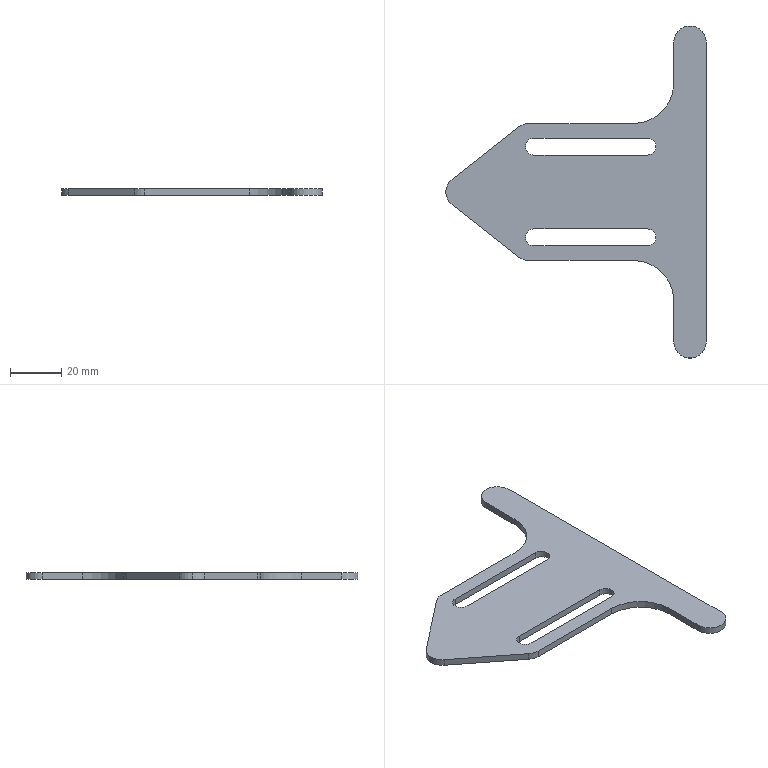Part | STEP file | GRM4_IMP_PLATE_64636-02_M | 1 solid | 27 faces | box 101.954 x 130.048 x 2.667 mm | volume 13683 mm3 | cylinder 14 | plane 13 | commonest cylinder face diameters 6.604 x6 12.7 x6 31.75 x2
STEP:
#1=CARTESIAN_POINT('',(3.964,0.,1.333));
#2=VERTEX_POINT('',#1);
#3=CARTESIAN_POINT('',(6.405,-5.004,1.333));
#4=VERTEX_POINT('',#3);
#5=CARTESIAN_POINT('',(10.314,0.,1.333));
#6=DIRECTION('',(0.,0.,1.));
#7=DIRECTION('',(-1.,0.,0.));
#8=AXIS2_PLACEMENT_3D('',#5,#6,#7);
#9=CIRCLE('',#8,6.35);
#10=EDGE_CURVE('',#2,#4,#9,.T.);
#11=ORIENTED_EDGE('',*,*,#10,.F.);
#12=CARTESIAN_POINT('',(3.964,0.,-1.333));
#13=VERTEX_POINT('',#12);
#14=CARTESIAN_POINT('',(3.964,0.,1.333));
#15=DIRECTION('',(0.,0.,-1.));
#16=VECTOR('',#15,1000.);
#17=LINE('',#14,#16);
#18=EDGE_CURVE('',#2,#13,#17,.T.);
#19=ORIENTED_EDGE('',*,*,#18,.T.);
#20=CARTESIAN_POINT('',(6.405,-5.004,-1.334));
#21=VERTEX_POINT('',#20);
#22=CARTESIAN_POINT('',(10.314,0.,-1.333));
#23=DIRECTION('',(0.,0.,1.));
#24=DIRECTION('',(-1.,0.,0.));
#25=AXIS2_PLACEMENT_3D('',#22,#23,#24);
#26=CIRCLE('',#25,6.35);
#27=EDGE_CURVE('',#13,#21,#26,.T.);
#28=ORIENTED_EDGE('',*,*,#27,.T.);
#29=CARTESIAN_POINT('',(6.405,-5.004,1.333));
#30=DIRECTION('',(0.,0.,1.));
#31=VECTOR('',#30,1000.);
#32=LINE('',#29,#31);
#33=EDGE_CURVE('',#21,#4,#32,.T.);
#34=ORIENTED_EDGE('',*,*,#33,.T.);
#35=EDGE_LOOP('',(#11,#19,#28,#34));
#36=FACE_OUTER_BOUND('',#35,.T.);
#37=CARTESIAN_POINT('',(10.314,0.,1.333));
#38=DIRECTION('',(0.,0.,-1.));
#39=DIRECTION('',(-1.,0.,0.));
#40=AXIS2_PLACEMENT_3D('',#37,#38,#39);
#41=CYLINDRICAL_SURFACE('',#40,6.35);
#42=ADVANCED_FACE('',(#36),#41,.T.);
#43=CARTESIAN_POINT('',(35.179,17.78,1.333));
#44=VERTEX_POINT('',#43);
#45=CARTESIAN_POINT('',(38.481,21.082,1.333));
#46=VERTEX_POINT('',#45);
#47=CARTESIAN_POINT('',(38.481,17.78,1.333));
#48=DIRECTION('',(0.,0.,-1.));
#49=DIRECTION('',(-1.,0.,0.));
#50=AXIS2_PLACEMENT_3D('',#47,#48,#49);
#51=CIRCLE('',#50,3.302);
#52=EDGE_CURVE('',#44,#46,#51,.T.);
#53=ORIENTED_EDGE('',*,*,#52,.F.);
#54=CARTESIAN_POINT('',(35.179,17.78,-1.333));
#55=VERTEX_POINT('',#54);
#56=CARTESIAN_POINT('',(35.179,17.78,1.333));
#57=DIRECTION('',(0.,0.,-1.));
#58=VECTOR('',#57,1000.);
#59=LINE('',#56,#58);
#60=EDGE_CURVE('',#44,#55,#59,.T.);
#61=ORIENTED_EDGE('',*,*,#60,.T.);
#62=CARTESIAN_POINT('',(38.481,21.082,-1.333));
#63=VERTEX_POINT('',#62);
#64=CARTESIAN_POINT('',(38.481,17.78,-1.333));
#65=DIRECTION('',(0.,0.,1.));
#66=DIRECTION('',(-1.,0.,0.));
#67=AXIS2_PLACEMENT_3D('',#64,#65,#66);
#68=CIRCLE('',#67,3.302);
#69=EDGE_CURVE('',#63,#55,#68,.T.);
#70=ORIENTED_EDGE('',*,*,#69,.F.);
#71=CARTESIAN_POINT('',(38.481,21.082,1.333));
#72=DIRECTION('',(0.,0.,-1.));
#73=VECTOR('',#72,1000.);
#74=LINE('',#71,#73);
#75=EDGE_CURVE('',#46,#63,#74,.T.);
#76=ORIENTED_EDGE('',*,*,#75,.F.);
#77=EDGE_LOOP('',(#53,#61,#70,#76));
#78=FACE_OUTER_BOUND('',#77,.T.);
#79=CARTESIAN_POINT('',(38.481,17.78,1.333));
#80=DIRECTION('',(0.,0.,-1.));
#81=DIRECTION('',(-1.,0.,0.));
#82=AXIS2_PLACEMENT_3D('',#79,#80,#81);
#83=CYLINDRICAL_SURFACE('',#82,3.302);
#84=ADVANCED_FACE('',(#78),#83,.F.);
#85=CARTESIAN_POINT('',(35.179,-17.78,1.333));
#86=VERTEX_POINT('',#85);
#87=CARTESIAN_POINT('',(38.481,-14.478,1.333));
#88=VERTEX_POINT('',#87);
#89=CARTESIAN_POINT('',(38.481,-17.78,1.333));
#90=DIRECTION('',(0.,0.,-1.));
#91=DIRECTION('',(-1.,0.,0.));
#92=AXIS2_PLACEMENT_3D('',#89,#90,#91);
#93=CIRCLE('',#92,3.302);
#94=EDGE_CURVE('',#86,#88,#93,.T.);
#95=ORIENTED_EDGE('',*,*,#94,.F.);
#96=CARTESIAN_POINT('',(35.179,-17.78,-1.333));
#97=VERTEX_POINT('',#96);
#98=CARTESIAN_POINT('',(35.179,-17.78,1.333));
#99=DIRECTION('',(0.,0.,-1.));
#100=VECTOR('',#99,1000.);
#101=LINE('',#98,#100);
#102=EDGE_CURVE('',#86,#97,#101,.T.);
#103=ORIENTED_EDGE('',*,*,#102,.T.);
#104=CARTESIAN_POINT('',(38.481,-14.478,-1.333));
#105=VERTEX_POINT('',#104);
#106=CARTESIAN_POINT('',(38.481,-17.78,-1.333));
#107=DIRECTION('',(0.,0.,1.));
#108=DIRECTION('',(-1.,0.,0.));
#109=AXIS2_PLACEMENT_3D('',#106,#107,#108);
#110=CIRCLE('',#109,3.302);
#111=EDGE_CURVE('',#105,#97,#110,.T.);
#112=ORIENTED_EDGE('',*,*,#111,.F.);
#113=CARTESIAN_POINT('',(38.481,-14.478,1.333));
#114=DIRECTION('',(0.,0.,-1.));
#115=VECTOR('',#114,1000.);
#116=LINE('',#113,#115);
#117=EDGE_CURVE('',#88,#105,#116,.T.);
#118=ORIENTED_EDGE('',*,*,#117,.F.);
#119=EDGE_LOOP('',(#95,#103,#112,#118));
#120=FACE_OUTER_BOUND('',#119,.T.);
#121=CARTESIAN_POINT('',(38.481,-17.78,1.333));
#122=DIRECTION('',(0.,0.,-1.));
#123=DIRECTION('',(-1.,0.,0.));
#124=AXIS2_PLACEMENT_3D('',#121,#122,#123);
#125=CYLINDRICAL_SURFACE('',#124,3.302);
#126=ADVANCED_FACE('',(#120),#125,.F.);
#127=CARTESIAN_POINT('',(77.343,26.797,1.333));
#128=VERTEX_POINT('',#127);
#129=CARTESIAN_POINT('',(36.485,26.797,1.333));
#130=VERTEX_POINT('',#129);
#131=CARTESIAN_POINT('',(10.314,26.797,1.333));
#132=DIRECTION('',(-1.,0.,0.));
#133=VECTOR('',#132,1000.);
#134=LINE('',#131,#133);
#135=EDGE_CURVE('',#128,#130,#134,.T.);
#136=ORIENTED_EDGE('',*,*,#135,.T.);
#137=CARTESIAN_POINT('',(32.576,25.451,1.333));
#138=VERTEX_POINT('',#137);
#139=CARTESIAN_POINT('',(36.485,20.447,1.333));
#140=DIRECTION('',(0.,0.,1.));
#141=DIRECTION('',(-1.,0.,0.));
#142=AXIS2_PLACEMENT_3D('',#139,#140,#141);
#143=CIRCLE('',#142,6.35);
#144=EDGE_CURVE('',#130,#138,#143,.T.);
#145=ORIENTED_EDGE('',*,*,#144,.T.);
#146=CARTESIAN_POINT('',(6.405,5.004,1.333));
#147=VERTEX_POINT('',#146);
#148=CARTESIAN_POINT('',(32.576,25.451,1.333));
#149=DIRECTION('',(-0.788,-0.6157,0.));
#150=VECTOR('',#149,1000.);
#151=LINE('',#148,#150);
#152=EDGE_CURVE('',#138,#147,#151,.T.);
#153=ORIENTED_EDGE('',*,*,#152,.T.);
#154=CARTESIAN_POINT('',(10.314,0.,1.333));
#155=DIRECTION('',(0.,0.,1.));
#156=DIRECTION('',(-1.,0.,0.));
#157=AXIS2_PLACEMENT_3D('',#154,#155,#156);
#158=CIRCLE('',#157,6.35);
#159=EDGE_CURVE('',#147,#2,#158,.T.);
#160=ORIENTED_EDGE('',*,*,#159,.T.);
#161=ORIENTED_EDGE('',*,*,#10,.T.);
#162=CARTESIAN_POINT('',(32.576,-25.451,1.333));
#163=VERTEX_POINT('',#162);
#164=CARTESIAN_POINT('',(6.405,-5.004,1.333));
#165=DIRECTION('',(0.788,-0.6157,0.));
#166=VECTOR('',#165,1000.);
#167=LINE('',#164,#166);
#168=EDGE_CURVE('',#4,#163,#167,.T.);
#169=ORIENTED_EDGE('',*,*,#168,.T.);
#170=CARTESIAN_POINT('',(36.485,-26.797,1.333));
#171=VERTEX_POINT('',#170);
#172=CARTESIAN_POINT('',(36.485,-20.447,1.333));
#173=DIRECTION('',(0.,0.,1.));
#174=DIRECTION('',(-1.,0.,0.));
#175=AXIS2_PLACEMENT_3D('',#172,#173,#174);
#176=CIRCLE('',#175,6.35);
#177=EDGE_CURVE('',#163,#171,#176,.T.);
#178=ORIENTED_EDGE('',*,*,#177,.T.);
#179=CARTESIAN_POINT('',(77.343,-26.797,1.333));
#180=VERTEX_POINT('',#179);
#181=CARTESIAN_POINT('',(10.314,-26.797,1.333));
#182=DIRECTION('',(1.,0.,0.));
#183=VECTOR('',#182,1000.);
#184=LINE('',#181,#183);
#185=EDGE_CURVE('',#171,#180,#184,.T.);
#186=ORIENTED_EDGE('',*,*,#185,.T.);
#187=CARTESIAN_POINT('',(93.218,-42.672,1.333));
#188=VERTEX_POINT('',#187);
#189=CARTESIAN_POINT('',(77.343,-42.672,1.333));
#190=DIRECTION('',(0.,0.,-1.));
#191=DIRECTION('',(-1.,0.,0.));
#192=AXIS2_PLACEMENT_3D('',#189,#190,#191);
#193=CIRCLE('',#192,15.875);
#194=EDGE_CURVE('',#180,#188,#193,.T.);
#195=ORIENTED_EDGE('',*,*,#194,.T.);
#196=CARTESIAN_POINT('',(93.218,-58.674,1.333));
#197=VERTEX_POINT('',#196);
#198=CARTESIAN_POINT('',(93.218,0.,1.333));
#199=DIRECTION('',(0.,-1.,0.));
#200=VECTOR('',#199,1000.);
#201=LINE('',#198,#200);
#202=EDGE_CURVE('',#188,#197,#201,.T.);
#203=ORIENTED_EDGE('',*,*,#202,.T.);
#204=CARTESIAN_POINT('',(105.918,-58.674,1.333));
#205=VERTEX_POINT('',#204);
#206=CARTESIAN_POINT('',(99.568,-58.674,1.333));
#207=DIRECTION('',(0.,0.,1.));
#208=DIRECTION('',(-1.,0.,0.));
#209=AXIS2_PLACEMENT_3D('',#206,#207,#208);
#210=CIRCLE('',#209,6.35);
#211=EDGE_CURVE('',#197,#205,#210,.T.);
#212=ORIENTED_EDGE('',*,*,#211,.T.);
#213=CARTESIAN_POINT('',(105.918,58.674,1.333));
#214=VERTEX_POINT('',#213);
#215=CARTESIAN_POINT('',(105.918,0.,1.333));
#216=DIRECTION('',(0.,1.,0.));
#217=VECTOR('',#216,1000.);
#218=LINE('',#215,#217);
#219=EDGE_CURVE('',#205,#214,#218,.T.);
#220=ORIENTED_EDGE('',*,*,#219,.T.);
#221=CARTESIAN_POINT('',(93.218,58.674,1.333));
#222=VERTEX_POINT('',#221);
#223=CARTESIAN_POINT('',(99.568,58.674,1.333));
#224=DIRECTION('',(0.,0.,1.));
#225=DIRECTION('',(-1.,0.,0.));
#226=AXIS2_PLACEMENT_3D('',#223,#224,#225);
#227=CIRCLE('',#226,6.35);
#228=EDGE_CURVE('',#214,#222,#227,.T.);
#229=ORIENTED_EDGE('',*,*,#228,.T.);
#230=CARTESIAN_POINT('',(93.218,42.672,1.333));
#231=VERTEX_POINT('',#230);
#232=CARTESIAN_POINT('',(93.218,0.,1.333));
#233=DIRECTION('',(0.,-1.,0.));
#234=VECTOR('',#233,1000.);
#235=LINE('',#232,#234);
#236=EDGE_CURVE('',#222,#231,#235,.T.);
#237=ORIENTED_EDGE('',*,*,#236,.T.);
#238=CARTESIAN_POINT('',(77.343,42.672,1.333));
#239=DIRECTION('',(0.,0.,-1.));
#240=DIRECTION('',(-1.,0.,0.));
#241=AXIS2_PLACEMENT_3D('',#238,#239,#240);
#242=CIRCLE('',#241,15.875);
#243=EDGE_CURVE('',#231,#128,#242,.T.);
#244=ORIENTED_EDGE('',*,*,#243,.T.);
#245=EDGE_LOOP('',(#136,#145,#153,#160,#161,#169,#178,#186,#195,#203,#212,#220,#229,#237,#244));
#246=FACE_OUTER_BOUND('',#245,.T.);
#247=CARTESIAN_POINT('',(82.931,14.478,1.333));
#248=VERTEX_POINT('',#247);
#249=CARTESIAN_POINT('',(38.481,14.478,1.333));
#250=VERTEX_POINT('',#249);
#251=CARTESIAN_POINT('',(10.314,14.478,1.333));
#252=DIRECTION('',(-1.,0.,0.));
#253=VECTOR('',#252,1000.);
#254=LINE('',#251,#253);
#255=EDGE_CURVE('',#248,#250,#254,.T.);
#256=ORIENTED_EDGE('',*,*,#255,.T.);
#257=CARTESIAN_POINT('',(38.481,17.78,1.333));
#258=DIRECTION('',(0.,0.,-1.));
#259=DIRECTION('',(-1.,0.,0.));
#260=AXIS2_PLACEMENT_3D('',#257,#258,#259);
#261=CIRCLE('',#260,3.302);
#262=EDGE_CURVE('',#250,#44,#261,.T.);
#263=ORIENTED_EDGE('',*,*,#262,.T.);
#264=ORIENTED_EDGE('',*,*,#52,.T.);
#265=CARTESIAN_POINT('',(82.931,21.082,1.333));
#266=VERTEX_POINT('',#265);
#267=CARTESIAN_POINT('',(10.314,21.082,1.333));
#268=DIRECTION('',(1.,0.,0.));
#269=VECTOR('',#268,1000.);
#270=LINE('',#267,#269);
#271=EDGE_CURVE('',#46,#266,#270,.T.);
#272=ORIENTED_EDGE('',*,*,#271,.T.);
#273=CARTESIAN_POINT('',(82.931,17.78,1.333));
#274=DIRECTION('',(0.,0.,-1.));
#275=DIRECTION('',(-1.,0.,0.));
#276=AXIS2_PLACEMENT_3D('',#273,#274,#275);
#277=CIRCLE('',#276,3.302);
#278=EDGE_CURVE('',#266,#248,#277,.T.);
#279=ORIENTED_EDGE('',*,*,#278,.T.);
#280=EDGE_LOOP('',(#256,#263,#264,#272,#279));
#281=FACE_BOUND('',#280,.T.);
#282=CARTESIAN_POINT('',(82.931,-21.082,1.333));
#283=VERTEX_POINT('',#282);
#284=CARTESIAN_POINT('',(38.481,-21.082,1.333));
#285=VERTEX_POINT('',#284);
#286=CARTESIAN_POINT('',(10.314,-21.082,1.333));
#287=DIRECTION('',(-1.,0.,0.));
#288=VECTOR('',#287,1000.);
#289=LINE('',#286,#288);
#290=EDGE_CURVE('',#283,#285,#289,.T.);
#291=ORIENTED_EDGE('',*,*,#290,.T.);
#292=CARTESIAN_POINT('',(38.481,-17.78,1.333));
#293=DIRECTION('',(0.,0.,-1.));
#294=DIRECTION('',(-1.,0.,0.));
#295=AXIS2_PLACEMENT_3D('',#292,#293,#294);
#296=CIRCLE('',#295,3.302);
#297=EDGE_CURVE('',#285,#86,#296,.T.);
#298=ORIENTED_EDGE('',*,*,#297,.T.);
#299=ORIENTED_EDGE('',*,*,#94,.T.);
#300=CARTESIAN_POINT('',(82.931,-14.478,1.333));
#301=VERTEX_POINT('',#300);
#302=CARTESIAN_POINT('',(10.314,-14.478,1.333));
#303=DIRECTION('',(1.,0.,0.));
#304=VECTOR('',#303,1000.);
#305=LINE('',#302,#304);
#306=EDGE_CURVE('',#88,#301,#305,.T.);
#307=ORIENTED_EDGE('',*,*,#306,.T.);
#308=CARTESIAN_POINT('',(82.931,-17.78,1.333));
#309=DIRECTION('',(0.,0.,-1.));
#310=DIRECTION('',(-1.,0.,0.));
#311=AXIS2_PLACEMENT_3D('',#308,#309,#310);
#312=CIRCLE('',#311,3.302);
#313=EDGE_CURVE('',#301,#283,#312,.T.);
#314=ORIENTED_EDGE('',*,*,#313,.T.);
#315=EDGE_LOOP('',(#291,#298,#299,#307,#314));
#316=FACE_BOUND('',#315,.T.);
#317=CARTESIAN_POINT('',(10.314,0.,1.333));
#318=DIRECTION('',(0.,0.,1.));
#319=DIRECTION('',(1.,0.,0.));
#320=AXIS2_PLACEMENT_3D('',#317,#318,#319);
#321=PLANE('',#320);
#322=ADVANCED_FACE('',(#246,#281,#316),#321,.T.);
#323=ORIENTED_EDGE('',*,*,#144,.F.);
#324=CARTESIAN_POINT('',(36.485,26.797,-1.333));
#325=VERTEX_POINT('',#324);
#326=CARTESIAN_POINT('',(36.485,26.797,1.333));
#327=DIRECTION('',(0.,0.,-1.));
#328=VECTOR('',#327,1000.);
#329=LINE('',#326,#328);
#330=EDGE_CURVE('',#130,#325,#329,.T.);
#331=ORIENTED_EDGE('',*,*,#330,.T.);
#332=CARTESIAN_POINT('',(32.576,25.451,-1.333));
#333=VERTEX_POINT('',#332);
#334=CARTESIAN_POINT('',(36.485,20.447,-1.333));
#335=DIRECTION('',(0.,0.,1.));
#336=DIRECTION('',(-1.,0.,0.));
#337=AXIS2_PLACEMENT_3D('',#334,#335,#336);
#338=CIRCLE('',#337,6.35);
#339=EDGE_CURVE('',#325,#333,#338,.T.);
#340=ORIENTED_EDGE('',*,*,#339,.T.);
#341=CARTESIAN_POINT('',(32.576,25.451,1.333));
#342=DIRECTION('',(0.,0.,1.));
#343=VECTOR('',#342,1000.);
#344=LINE('',#341,#343);
#345=EDGE_CURVE('',#333,#138,#344,.T.);
#346=ORIENTED_EDGE('',*,*,#345,.T.);
#347=EDGE_LOOP('',(#323,#331,#340,#346));
#348=FACE_OUTER_BOUND('',#347,.T.);
#349=CARTESIAN_POINT('',(36.485,20.447,1.333));
#350=DIRECTION('',(0.,0.,-1.));
#351=DIRECTION('',(-1.,0.,0.));
#352=AXIS2_PLACEMENT_3D('',#349,#350,#351);
#353=CYLINDRICAL_SURFACE('',#352,6.35);
#354=ADVANCED_FACE('',(#348),#353,.T.);
#355=ORIENTED_EDGE('',*,*,#330,.F.);
#356=ORIENTED_EDGE('',*,*,#135,.F.);
#357=CARTESIAN_POINT('',(77.343,26.797,-1.333));
#358=VERTEX_POINT('',#357);
#359=CARTESIAN_POINT('',(77.343,26.797,1.333));
#360=DIRECTION('',(0.,0.,1.));
#361=VECTOR('',#360,1000.);
#362=LINE('',#359,#361);
#363=EDGE_CURVE('',#358,#128,#362,.T.);
#364=ORIENTED_EDGE('',*,*,#363,.F.);
#365=CARTESIAN_POINT('',(77.343,26.797,-1.333));
#366=DIRECTION('',(1.,0.,0.));
#367=VECTOR('',#366,1000.);
#368=LINE('',#365,#367);
#369=EDGE_CURVE('',#325,#358,#368,.T.);
#370=ORIENTED_EDGE('',*,*,#369,.F.);
#371=EDGE_LOOP('',(#355,#356,#364,#370));
#372=FACE_OUTER_BOUND('',#371,.T.);
#373=CARTESIAN_POINT('',(77.343,26.797,1.333));
#374=DIRECTION('',(0.,-1.,0.));
#375=DIRECTION('',(0.,0.,-1.));
#376=AXIS2_PLACEMENT_3D('',#373,#374,#375);
#377=PLANE('',#376);
#378=ADVANCED_FACE('',(#372),#377,.F.);
#379=ORIENTED_EDGE('',*,*,#363,.T.);
#380=ORIENTED_EDGE('',*,*,#243,.F.);
#381=CARTESIAN_POINT('',(93.218,42.672,-1.333));
#382=VERTEX_POINT('',#381);
#383=CARTESIAN_POINT('',(93.218,42.672,1.333));
#384=DIRECTION('',(0.,0.,1.));
#385=VECTOR('',#384,1000.);
#386=LINE('',#383,#385);
#387=EDGE_CURVE('',#382,#231,#386,.T.);
#388=ORIENTED_EDGE('',*,*,#387,.F.);
#389=CARTESIAN_POINT('',(77.343,42.672,-1.333));
#390=DIRECTION('',(0.,0.,1.));
#391=DIRECTION('',(-1.,0.,0.));
#392=AXIS2_PLACEMENT_3D('',#389,#390,#391);
#393=CIRCLE('',#392,15.875);
#394=EDGE_CURVE('',#358,#382,#393,.T.);
#395=ORIENTED_EDGE('',*,*,#394,.F.);
#396=EDGE_LOOP('',(#379,#380,#388,#395));
#397=FACE_OUTER_BOUND('',#396,.T.);
#398=CARTESIAN_POINT('',(77.343,42.672,1.333));
#399=DIRECTION('',(0.,0.,-1.));
#400=DIRECTION('',(-1.,0.,0.));
#401=AXIS2_PLACEMENT_3D('',#398,#399,#400);
#402=CYLINDRICAL_SURFACE('',#401,15.875);
#403=ADVANCED_FACE('',(#397),#402,.F.);
#404=ORIENTED_EDGE('',*,*,#387,.T.);
#405=ORIENTED_EDGE('',*,*,#236,.F.);
#406=CARTESIAN_POINT('',(93.218,58.674,-1.333));
#407=VERTEX_POINT('',#406);
#408=CARTESIAN_POINT('',(93.218,58.674,1.333));
#409=DIRECTION('',(0.,0.,1.));
#410=VECTOR('',#409,1000.);
#411=LINE('',#408,#410);
#412=EDGE_CURVE('',#407,#222,#411,.T.);
#413=ORIENTED_EDGE('',*,*,#412,.F.);
#414=CARTESIAN_POINT('',(93.218,58.674,-1.333));
#415=DIRECTION('',(0.,1.,0.));
#416=VECTOR('',#415,1000.);
#417=LINE('',#414,#416);
#418=EDGE_CURVE('',#382,#407,#417,.T.);
#419=ORIENTED_EDGE('',*,*,#418,.F.);
#420=EDGE_LOOP('',(#404,#405,#413,#419));
#421=FACE_OUTER_BOUND('',#420,.T.);
#422=CARTESIAN_POINT('',(93.218,58.674,1.333));
#423=DIRECTION('',(1.,0.,0.));
#424=DIRECTION('',(0.,0.,-1.));
#425=AXIS2_PLACEMENT_3D('',#422,#423,#424);
#426=PLANE('',#425);
#427=ADVANCED_FACE('',(#421),#426,.F.);
#428=ORIENTED_EDGE('',*,*,#228,.F.);
#429=CARTESIAN_POINT('',(105.918,58.674,-1.333));
#430=VERTEX_POINT('',#429);
#431=CARTESIAN_POINT('',(105.918,58.674,1.333));
#432=DIRECTION('',(0.,0.,-1.));
#433=VECTOR('',#432,1000.);
#434=LINE('',#431,#433);
#435=EDGE_CURVE('',#214,#430,#434,.T.);
#436=ORIENTED_EDGE('',*,*,#435,.T.);
#437=CARTESIAN_POINT('',(99.568,58.674,-1.333));
#438=DIRECTION('',(0.,0.,1.));
#439=DIRECTION('',(-1.,0.,0.));
#440=AXIS2_PLACEMENT_3D('',#437,#438,#439);
#441=CIRCLE('',#440,6.35);
#442=EDGE_CURVE('',#430,#407,#441,.T.);
#443=ORIENTED_EDGE('',*,*,#442,.T.);
#444=ORIENTED_EDGE('',*,*,#412,.T.);
#445=EDGE_LOOP('',(#428,#436,#443,#444));
#446=FACE_OUTER_BOUND('',#445,.T.);
#447=CARTESIAN_POINT('',(99.568,58.674,1.333));
#448=DIRECTION('',(0.,0.,-1.));
#449=DIRECTION('',(-1.,0.,0.));
#450=AXIS2_PLACEMENT_3D('',#447,#448,#449);
#451=CYLINDRICAL_SURFACE('',#450,6.35);
#452=ADVANCED_FACE('',(#446),#451,.T.);
#453=ORIENTED_EDGE('',*,*,#435,.F.);
#454=ORIENTED_EDGE('',*,*,#219,.F.);
#455=CARTESIAN_POINT('',(105.918,-58.674,-1.333));
#456=VERTEX_POINT('',#455);
#457=CARTESIAN_POINT('',(105.918,-58.674,1.333));
#458=DIRECTION('',(0.,0.,1.));
#459=VECTOR('',#458,1000.);
#460=LINE('',#457,#459);
#461=EDGE_CURVE('',#456,#205,#460,.T.);
#462=ORIENTED_EDGE('',*,*,#461,.F.);
#463=CARTESIAN_POINT('',(105.918,-58.674,-1.333));
#464=DIRECTION('',(0.,-1.,0.));
#465=VECTOR('',#464,1000.);
#466=LINE('',#463,#465);
#467=EDGE_CURVE('',#430,#456,#466,.T.);
#468=ORIENTED_EDGE('',*,*,#467,.F.);
#469=EDGE_LOOP('',(#453,#454,#462,#468));
#470=FACE_OUTER_BOUND('',#469,.T.);
#471=CARTESIAN_POINT('',(105.918,-58.674,1.333));
#472=DIRECTION('',(-1.,0.,0.));
#473=DIRECTION('',(0.,0.,1.));
#474=AXIS2_PLACEMENT_3D('',#471,#472,#473);
#475=PLANE('',#474);
#476=ADVANCED_FACE('',(#470),#475,.F.);
#477=ORIENTED_EDGE('',*,*,#211,.F.);
#478=CARTESIAN_POINT('',(93.218,-58.674,-1.333));
#479=VERTEX_POINT('',#478);
#480=CARTESIAN_POINT('',(93.218,-58.674,1.333));
#481=DIRECTION('',(0.,0.,-1.));
#482=VECTOR('',#481,1000.);
#483=LINE('',#480,#482);
#484=EDGE_CURVE('',#197,#479,#483,.T.);
#485=ORIENTED_EDGE('',*,*,#484,.T.);
#486=CARTESIAN_POINT('',(99.568,-58.674,-1.333));
#487=DIRECTION('',(0.,0.,1.));
#488=DIRECTION('',(-1.,0.,0.));
#489=AXIS2_PLACEMENT_3D('',#486,#487,#488);
#490=CIRCLE('',#489,6.35);
#491=EDGE_CURVE('',#479,#456,#490,.T.);
#492=ORIENTED_EDGE('',*,*,#491,.T.);
#493=ORIENTED_EDGE('',*,*,#461,.T.);
#494=EDGE_LOOP('',(#477,#485,#492,#493));
#495=FACE_OUTER_BOUND('',#494,.T.);
#496=CARTESIAN_POINT('',(99.568,-58.674,1.333));
#497=DIRECTION('',(0.,0.,-1.));
#498=DIRECTION('',(-1.,0.,0.));
#499=AXIS2_PLACEMENT_3D('',#496,#497,#498);
#500=CYLINDRICAL_SURFACE('',#499,6.35);
#501=ADVANCED_FACE('',(#495),#500,.T.);
#502=ORIENTED_EDGE('',*,*,#484,.F.);
#503=ORIENTED_EDGE('',*,*,#202,.F.);
#504=CARTESIAN_POINT('',(93.218,-42.672,-1.333));
#505=VERTEX_POINT('',#504);
#506=CARTESIAN_POINT('',(93.218,-42.672,1.333));
#507=DIRECTION('',(0.,0.,1.));
#508=VECTOR('',#507,1000.);
#509=LINE('',#506,#508);
#510=EDGE_CURVE('',#505,#188,#509,.T.);
#511=ORIENTED_EDGE('',*,*,#510,.F.);
#512=CARTESIAN_POINT('',(93.218,-42.672,-1.333));
#513=DIRECTION('',(0.,1.,0.));
#514=VECTOR('',#513,1000.);
#515=LINE('',#512,#514);
#516=EDGE_CURVE('',#479,#505,#515,.T.);
#517=ORIENTED_EDGE('',*,*,#516,.F.);
#518=EDGE_LOOP('',(#502,#503,#511,#517));
#519=FACE_OUTER_BOUND('',#518,.T.);
#520=CARTESIAN_POINT('',(93.218,-42.672,1.333));
#521=DIRECTION('',(1.,0.,0.));
#522=DIRECTION('',(0.,0.,-1.));
#523=AXIS2_PLACEMENT_3D('',#520,#521,#522);
#524=PLANE('',#523);
#525=ADVANCED_FACE('',(#519),#524,.F.);
#526=ORIENTED_EDGE('',*,*,#510,.T.);
#527=ORIENTED_EDGE('',*,*,#194,.F.);
#528=CARTESIAN_POINT('',(77.343,-26.797,-1.333));
#529=VERTEX_POINT('',#528);
#530=CARTESIAN_POINT('',(77.343,-26.797,1.333));
#531=DIRECTION('',(0.,0.,1.));
#532=VECTOR('',#531,1000.);
#533=LINE('',#530,#532);
#534=EDGE_CURVE('',#529,#180,#533,.T.);
#535=ORIENTED_EDGE('',*,*,#534,.F.);
#536=CARTESIAN_POINT('',(77.343,-42.672,-1.333));
#537=DIRECTION('',(0.,0.,1.));
#538=DIRECTION('',(-1.,0.,0.));
#539=AXIS2_PLACEMENT_3D('',#536,#537,#538);
#540=CIRCLE('',#539,15.875);
#541=EDGE_CURVE('',#505,#529,#540,.T.);
#542=ORIENTED_EDGE('',*,*,#541,.F.);
#543=EDGE_LOOP('',(#526,#527,#535,#542));
#544=FACE_OUTER_BOUND('',#543,.T.);
#545=CARTESIAN_POINT('',(77.343,-42.672,1.333));
#546=DIRECTION('',(0.,0.,-1.));
#547=DIRECTION('',(-1.,0.,0.));
#548=AXIS2_PLACEMENT_3D('',#545,#546,#547);
#549=CYLINDRICAL_SURFACE('',#548,15.875);
#550=ADVANCED_FACE('',(#544),#549,.F.);
#551=ORIENTED_EDGE('',*,*,#534,.T.);
#552=ORIENTED_EDGE('',*,*,#185,.F.);
#553=CARTESIAN_POINT('',(36.485,-26.797,-1.333));
#554=VERTEX_POINT('',#553);
#555=CARTESIAN_POINT('',(36.485,-26.797,1.333));
#556=DIRECTION('',(0.,0.,1.));
#557=VECTOR('',#556,1000.);
#558=LINE('',#555,#557);
#559=EDGE_CURVE('',#554,#171,#558,.T.);
#560=ORIENTED_EDGE('',*,*,#559,.F.);
#561=CARTESIAN_POINT('',(36.485,-26.797,-1.333));
#562=DIRECTION('',(-1.,0.,0.));
#563=VECTOR('',#562,1000.);
#564=LINE('',#561,#563);
#565=EDGE_CURVE('',#529,#554,#564,.T.);
#566=ORIENTED_EDGE('',*,*,#565,.F.);
#567=EDGE_LOOP('',(#551,#552,#560,#566));
#568=FACE_OUTER_BOUND('',#567,.T.);
#569=CARTESIAN_POINT('',(36.485,-26.797,1.333));
#570=DIRECTION('',(0.,1.,0.));
#571=DIRECTION('',(0.,0.,1.));
#572=AXIS2_PLACEMENT_3D('',#569,#570,#571);
#573=PLANE('',#572);
#574=ADVANCED_FACE('',(#568),#573,.F.);
#575=ORIENTED_EDGE('',*,*,#177,.F.);
#576=CARTESIAN_POINT('',(32.576,-25.451,-1.333));
#577=VERTEX_POINT('',#576);
#578=CARTESIAN_POINT('',(32.576,-25.451,1.333));
#579=DIRECTION('',(0.,0.,-1.));
#580=VECTOR('',#579,1000.);
#581=LINE('',#578,#580);
#582=EDGE_CURVE('',#163,#577,#581,.T.);
#583=ORIENTED_EDGE('',*,*,#582,.T.);
#584=CARTESIAN_POINT('',(36.485,-20.447,-1.333));
#585=DIRECTION('',(0.,0.,1.));
#586=DIRECTION('',(-1.,0.,0.));
#587=AXIS2_PLACEMENT_3D('',#584,#585,#586);
#588=CIRCLE('',#587,6.35);
#589=EDGE_CURVE('',#577,#554,#588,.T.);
#590=ORIENTED_EDGE('',*,*,#589,.T.);
#591=ORIENTED_EDGE('',*,*,#559,.T.);
#592=EDGE_LOOP('',(#575,#583,#590,#591));
#593=FACE_OUTER_BOUND('',#592,.T.);
#594=CARTESIAN_POINT('',(36.485,-20.447,1.333));
#595=DIRECTION('',(0.,0.,-1.));
#596=DIRECTION('',(-1.,0.,0.));
#597=AXIS2_PLACEMENT_3D('',#594,#595,#596);
#598=CYLINDRICAL_SURFACE('',#597,6.35);
#599=ADVANCED_FACE('',(#593),#598,.T.);
#600=ORIENTED_EDGE('',*,*,#582,.F.);
#601=ORIENTED_EDGE('',*,*,#168,.F.);
#602=ORIENTED_EDGE('',*,*,#33,.F.);
#603=CARTESIAN_POINT('',(6.405,-5.004,-1.334));
#604=DIRECTION('',(-0.788,0.6157,0.));
#605=VECTOR('',#604,1000.);
#606=LINE('',#603,#605);
#607=EDGE_CURVE('',#577,#21,#606,.T.);
#608=ORIENTED_EDGE('',*,*,#607,.F.);
#609=EDGE_LOOP('',(#600,#601,#602,#608));
#610=FACE_OUTER_BOUND('',#609,.T.);
#611=CARTESIAN_POINT('',(6.405,-5.004,1.333));
#612=DIRECTION('',(0.6157,0.788,0.));
#613=DIRECTION('',(-0.788,0.6157,0.));
#614=AXIS2_PLACEMENT_3D('',#611,#612,#613);
#615=PLANE('',#614);
#616=ADVANCED_FACE('',(#610),#615,.F.);
#617=ORIENTED_EDGE('',*,*,#18,.F.);
#618=ORIENTED_EDGE('',*,*,#159,.F.);
#619=CARTESIAN_POINT('',(6.405,5.004,-1.333));
#620=VERTEX_POINT('',#619);
#621=CARTESIAN_POINT('',(6.405,5.004,1.333));
#622=DIRECTION('',(0.,0.,-1.));
#623=VECTOR('',#622,1000.);
#624=LINE('',#621,#623);
#625=EDGE_CURVE('',#147,#620,#624,.T.);
#626=ORIENTED_EDGE('',*,*,#625,.T.);
#627=CARTESIAN_POINT('',(10.314,0.,-1.333));
#628=DIRECTION('',(0.,0.,1.));
#629=DIRECTION('',(-1.,0.,0.));
#630=AXIS2_PLACEMENT_3D('',#627,#628,#629);
#631=CIRCLE('',#630,6.35);
#632=EDGE_CURVE('',#620,#13,#631,.T.);
#633=ORIENTED_EDGE('',*,*,#632,.T.);
#634=EDGE_LOOP('',(#617,#618,#626,#633));
#635=FACE_OUTER_BOUND('',#634,.T.);
#636=CARTESIAN_POINT('',(10.314,0.,1.333));
#637=DIRECTION('',(0.,0.,-1.));
#638=DIRECTION('',(-1.,0.,0.));
#639=AXIS2_PLACEMENT_3D('',#636,#637,#638);
#640=CYLINDRICAL_SURFACE('',#639,6.35);
#641=ADVANCED_FACE('',(#635),#640,.T.);
#642=ORIENTED_EDGE('',*,*,#625,.F.);
#643=ORIENTED_EDGE('',*,*,#152,.F.);
#644=ORIENTED_EDGE('',*,*,#345,.F.);
#645=CARTESIAN_POINT('',(32.576,25.451,-1.334));
#646=DIRECTION('',(0.788,0.6157,0.));
#647=VECTOR('',#646,1000.);
#648=LINE('',#645,#647);
#649=EDGE_CURVE('',#620,#333,#648,.T.);
#650=ORIENTED_EDGE('',*,*,#649,.F.);
#651=EDGE_LOOP('',(#642,#643,#644,#650));
#652=FACE_OUTER_BOUND('',#651,.T.);
#653=CARTESIAN_POINT('',(32.576,25.451,1.333));
#654=DIRECTION('',(0.6157,-0.788,0.));
#655=DIRECTION('',(0.788,0.6157,0.));
#656=AXIS2_PLACEMENT_3D('',#653,#654,#655);
#657=PLANE('',#656);
#658=ADVANCED_FACE('',(#652),#657,.F.);
#659=ORIENTED_EDGE('',*,*,#60,.F.);
#660=ORIENTED_EDGE('',*,*,#262,.F.);
#661=CARTESIAN_POINT('',(38.481,14.478,-1.333));
#662=VERTEX_POINT('',#661);
#663=CARTESIAN_POINT('',(38.481,14.478,1.333));
#664=DIRECTION('',(0.,0.,1.));
#665=VECTOR('',#664,1000.);
#666=LINE('',#663,#665);
#667=EDGE_CURVE('',#662,#250,#666,.T.);
#668=ORIENTED_EDGE('',*,*,#667,.F.);
#669=CARTESIAN_POINT('',(38.481,17.78,-1.333));
#670=DIRECTION('',(0.,0.,1.));
#671=DIRECTION('',(-1.,0.,0.));
#672=AXIS2_PLACEMENT_3D('',#669,#670,#671);
#673=CIRCLE('',#672,3.302);
#674=EDGE_CURVE('',#55,#662,#673,.T.);
#675=ORIENTED_EDGE('',*,*,#674,.F.);
#676=EDGE_LOOP('',(#659,#660,#668,#675));
#677=FACE_OUTER_BOUND('',#676,.T.);
#678=CARTESIAN_POINT('',(38.481,17.78,1.333));
#679=DIRECTION('',(0.,0.,-1.));
#680=DIRECTION('',(-1.,0.,0.));
#681=AXIS2_PLACEMENT_3D('',#678,#679,#680);
#682=CYLINDRICAL_SURFACE('',#681,3.302);
#683=ADVANCED_FACE('',(#677),#682,.F.);
#684=ORIENTED_EDGE('',*,*,#255,.F.);
#685=CARTESIAN_POINT('',(82.931,14.478,-1.333));
#686=VERTEX_POINT('',#685);
#687=CARTESIAN_POINT('',(82.931,14.478,1.333));
#688=DIRECTION('',(0.,0.,-1.));
#689=VECTOR('',#688,1000.);
#690=LINE('',#687,#689);
#691=EDGE_CURVE('',#248,#686,#690,.T.);
#692=ORIENTED_EDGE('',*,*,#691,.T.);
#693=CARTESIAN_POINT('',(38.481,14.478,-1.333));
#694=DIRECTION('',(-1.,0.,0.));
#695=VECTOR('',#694,1000.);
#696=LINE('',#693,#695);
#697=EDGE_CURVE('',#686,#662,#696,.T.);
#698=ORIENTED_EDGE('',*,*,#697,.T.);
#699=ORIENTED_EDGE('',*,*,#667,.T.);
#700=EDGE_LOOP('',(#684,#692,#698,#699));
#701=FACE_OUTER_BOUND('',#700,.T.);
#702=CARTESIAN_POINT('',(38.481,14.478,1.333));
#703=DIRECTION('',(0.,1.,0.));
#704=DIRECTION('',(0.,0.,1.));
#705=AXIS2_PLACEMENT_3D('',#702,#703,#704);
#706=PLANE('',#705);
#707=ADVANCED_FACE('',(#701),#706,.T.);
#708=ORIENTED_EDGE('',*,*,#691,.F.);
#709=ORIENTED_EDGE('',*,*,#278,.F.);
#710=CARTESIAN_POINT('',(82.931,21.082,-1.333));
#711=VERTEX_POINT('',#710);
#712=CARTESIAN_POINT('',(82.931,21.082,1.333));
#713=DIRECTION('',(0.,0.,1.));
#714=VECTOR('',#713,1000.);
#715=LINE('',#712,#714);
#716=EDGE_CURVE('',#711,#266,#715,.T.);
#717=ORIENTED_EDGE('',*,*,#716,.F.);
#718=CARTESIAN_POINT('',(82.931,17.78,-1.333));
#719=DIRECTION('',(0.,0.,1.));
#720=DIRECTION('',(-1.,0.,0.));
#721=AXIS2_PLACEMENT_3D('',#718,#719,#720);
#722=CIRCLE('',#721,3.302);
#723=EDGE_CURVE('',#686,#711,#722,.T.);
#724=ORIENTED_EDGE('',*,*,#723,.F.);
#725=EDGE_LOOP('',(#708,#709,#717,#724));
#726=FACE_OUTER_BOUND('',#725,.T.);
#727=CARTESIAN_POINT('',(82.931,17.78,1.333));
#728=DIRECTION('',(0.,0.,-1.));
#729=DIRECTION('',(-1.,0.,0.));
#730=AXIS2_PLACEMENT_3D('',#727,#728,#729);
#731=CYLINDRICAL_SURFACE('',#730,3.302);
#732=ADVANCED_FACE('',(#726),#731,.F.);
#733=ORIENTED_EDGE('',*,*,#271,.F.);
#734=ORIENTED_EDGE('',*,*,#75,.T.);
#735=CARTESIAN_POINT('',(82.931,21.082,-1.333));
#736=DIRECTION('',(1.,0.,0.));
#737=VECTOR('',#736,1000.);
#738=LINE('',#735,#737);
#739=EDGE_CURVE('',#63,#711,#738,.T.);
#740=ORIENTED_EDGE('',*,*,#739,.T.);
#741=ORIENTED_EDGE('',*,*,#716,.T.);
#742=EDGE_LOOP('',(#733,#734,#740,#741));
#743=FACE_OUTER_BOUND('',#742,.T.);
#744=CARTESIAN_POINT('',(82.931,21.082,1.333));
#745=DIRECTION('',(0.,-1.,0.));
#746=DIRECTION('',(0.,0.,-1.));
#747=AXIS2_PLACEMENT_3D('',#744,#745,#746);
#748=PLANE('',#747);
#749=ADVANCED_FACE('',(#743),#748,.T.);
#750=ORIENTED_EDGE('',*,*,#102,.F.);
#751=ORIENTED_EDGE('',*,*,#297,.F.);
#752=CARTESIAN_POINT('',(38.481,-21.082,-1.333));
#753=VERTEX_POINT('',#752);
#754=CARTESIAN_POINT('',(38.481,-21.082,1.333));
#755=DIRECTION('',(0.,0.,1.));
#756=VECTOR('',#755,1000.);
#757=LINE('',#754,#756);
#758=EDGE_CURVE('',#753,#285,#757,.T.);
#759=ORIENTED_EDGE('',*,*,#758,.F.);
#760=CARTESIAN_POINT('',(38.481,-17.78,-1.333));
#761=DIRECTION('',(0.,0.,1.));
#762=DIRECTION('',(-1.,0.,0.));
#763=AXIS2_PLACEMENT_3D('',#760,#761,#762);
#764=CIRCLE('',#763,3.302);
#765=EDGE_CURVE('',#97,#753,#764,.T.);
#766=ORIENTED_EDGE('',*,*,#765,.F.);
#767=EDGE_LOOP('',(#750,#751,#759,#766));
#768=FACE_OUTER_BOUND('',#767,.T.);
#769=CARTESIAN_POINT('',(38.481,-17.78,1.333));
#770=DIRECTION('',(0.,0.,-1.));
#771=DIRECTION('',(-1.,0.,0.));
#772=AXIS2_PLACEMENT_3D('',#769,#770,#771);
#773=CYLINDRICAL_SURFACE('',#772,3.302);
#774=ADVANCED_FACE('',(#768),#773,.F.);
#775=ORIENTED_EDGE('',*,*,#290,.F.);
#776=CARTESIAN_POINT('',(82.931,-21.082,-1.333));
#777=VERTEX_POINT('',#776);
#778=CARTESIAN_POINT('',(82.931,-21.082,1.333));
#779=DIRECTION('',(0.,0.,-1.));
#780=VECTOR('',#779,1000.);
#781=LINE('',#778,#780);
#782=EDGE_CURVE('',#283,#777,#781,.T.);
#783=ORIENTED_EDGE('',*,*,#782,.T.);
#784=CARTESIAN_POINT('',(38.481,-21.082,-1.333));
#785=DIRECTION('',(-1.,0.,0.));
#786=VECTOR('',#785,1000.);
#787=LINE('',#784,#786);
#788=EDGE_CURVE('',#777,#753,#787,.T.);
#789=ORIENTED_EDGE('',*,*,#788,.T.);
#790=ORIENTED_EDGE('',*,*,#758,.T.);
#791=EDGE_LOOP('',(#775,#783,#789,#790));
#792=FACE_OUTER_BOUND('',#791,.T.);
#793=CARTESIAN_POINT('',(38.481,-21.082,1.333));
#794=DIRECTION('',(0.,1.,0.));
#795=DIRECTION('',(0.,0.,1.));
#796=AXIS2_PLACEMENT_3D('',#793,#794,#795);
#797=PLANE('',#796);
#798=ADVANCED_FACE('',(#792),#797,.T.);
#799=ORIENTED_EDGE('',*,*,#782,.F.);
#800=ORIENTED_EDGE('',*,*,#313,.F.);
#801=CARTESIAN_POINT('',(82.931,-14.478,-1.333));
#802=VERTEX_POINT('',#801);
#803=CARTESIAN_POINT('',(82.931,-14.478,1.333));
#804=DIRECTION('',(0.,0.,1.));
#805=VECTOR('',#804,1000.);
#806=LINE('',#803,#805);
#807=EDGE_CURVE('',#802,#301,#806,.T.);
#808=ORIENTED_EDGE('',*,*,#807,.F.);
#809=CARTESIAN_POINT('',(82.931,-17.78,-1.333));
#810=DIRECTION('',(0.,0.,1.));
#811=DIRECTION('',(-1.,0.,0.));
#812=AXIS2_PLACEMENT_3D('',#809,#810,#811);
#813=CIRCLE('',#812,3.302);
#814=EDGE_CURVE('',#777,#802,#813,.T.);
#815=ORIENTED_EDGE('',*,*,#814,.F.);
#816=EDGE_LOOP('',(#799,#800,#808,#815));
#817=FACE_OUTER_BOUND('',#816,.T.);
#818=CARTESIAN_POINT('',(82.931,-17.78,1.333));
#819=DIRECTION('',(0.,0.,-1.));
#820=DIRECTION('',(-1.,0.,0.));
#821=AXIS2_PLACEMENT_3D('',#818,#819,#820);
#822=CYLINDRICAL_SURFACE('',#821,3.302);
#823=ADVANCED_FACE('',(#817),#822,.F.);
#824=ORIENTED_EDGE('',*,*,#306,.F.);
#825=ORIENTED_EDGE('',*,*,#117,.T.);
#826=CARTESIAN_POINT('',(82.931,-14.478,-1.333));
#827=DIRECTION('',(1.,0.,0.));
#828=VECTOR('',#827,1000.);
#829=LINE('',#826,#828);
#830=EDGE_CURVE('',#105,#802,#829,.T.);
#831=ORIENTED_EDGE('',*,*,#830,.T.);
#832=ORIENTED_EDGE('',*,*,#807,.T.);
#833=EDGE_LOOP('',(#824,#825,#831,#832));
#834=FACE_OUTER_BOUND('',#833,.T.);
#835=CARTESIAN_POINT('',(82.931,-14.478,1.333));
#836=DIRECTION('',(0.,-1.,0.));
#837=DIRECTION('',(0.,0.,-1.));
#838=AXIS2_PLACEMENT_3D('',#835,#836,#837);
#839=PLANE('',#838);
#840=ADVANCED_FACE('',(#834),#839,.T.);
#841=ORIENTED_EDGE('',*,*,#339,.F.);
#842=ORIENTED_EDGE('',*,*,#369,.T.);
#843=ORIENTED_EDGE('',*,*,#394,.T.);
#844=ORIENTED_EDGE('',*,*,#418,.T.);
#845=ORIENTED_EDGE('',*,*,#442,.F.);
#846=ORIENTED_EDGE('',*,*,#467,.T.);
#847=ORIENTED_EDGE('',*,*,#491,.F.);
#848=ORIENTED_EDGE('',*,*,#516,.T.);
#849=ORIENTED_EDGE('',*,*,#541,.T.);
#850=ORIENTED_EDGE('',*,*,#565,.T.);
#851=ORIENTED_EDGE('',*,*,#589,.F.);
#852=ORIENTED_EDGE('',*,*,#607,.T.);
#853=ORIENTED_EDGE('',*,*,#27,.F.);
#854=ORIENTED_EDGE('',*,*,#632,.F.);
#855=ORIENTED_EDGE('',*,*,#649,.T.);
#856=EDGE_LOOP('',(#841,#842,#843,#844,#845,#846,#847,#848,#849,#850,#851,#852,#853,#854,#855));
#857=FACE_OUTER_BOUND('',#856,.T.);
#858=ORIENTED_EDGE('',*,*,#69,.T.);
#859=ORIENTED_EDGE('',*,*,#674,.T.);
#860=ORIENTED_EDGE('',*,*,#697,.F.);
#861=ORIENTED_EDGE('',*,*,#723,.T.);
#862=ORIENTED_EDGE('',*,*,#739,.F.);
#863=EDGE_LOOP('',(#858,#859,#860,#861,#862));
#864=FACE_BOUND('',#863,.T.);
#865=ORIENTED_EDGE('',*,*,#111,.T.);
#866=ORIENTED_EDGE('',*,*,#765,.T.);
#867=ORIENTED_EDGE('',*,*,#788,.F.);
#868=ORIENTED_EDGE('',*,*,#814,.T.);
#869=ORIENTED_EDGE('',*,*,#830,.F.);
#870=EDGE_LOOP('',(#865,#866,#867,#868,#869));
#871=FACE_BOUND('',#870,.T.);
#872=CARTESIAN_POINT('',(10.314,0.,-1.333));
#873=DIRECTION('',(0.,0.,1.));
#874=DIRECTION('',(1.,0.,0.));
#875=AXIS2_PLACEMENT_3D('',#872,#873,#874);
#876=PLANE('',#875);
#877=ADVANCED_FACE('',(#857,#864,#871),#876,.F.);
#878=CLOSED_SHELL('',(#42,#84,#126,#322,#354,#378,#403,#427,#452,#476,#501,#525,#550,#574,#599,#616,#641,#658,#683,#707,#732,#749,#774,#798,#823,#840,#877));
#879=MANIFOLD_SOLID_BREP('',#878);
#880=CARTESIAN_POINT('',(0.,0.,0.));
#881=DIRECTION('',(0.,0.,1.));
#882=DIRECTION('',(1.,0.,0.));
#883=AXIS2_PLACEMENT_3D('',#880,#881,#882);
#884=(LENGTH_UNIT()NAMED_UNIT(*)SI_UNIT(.MILLI.,.METRE.));
#885=UNCERTAINTY_MEASURE_WITH_UNIT(LENGTH_MEASURE(0.00001),#884,'','');
#886=(NAMED_UNIT(*)PLANE_ANGLE_UNIT()SI_UNIT($,.RADIAN.));
#887=(NAMED_UNIT(*)SI_UNIT($,.STERADIAN.)SOLID_ANGLE_UNIT());
#888=(GEOMETRIC_REPRESENTATION_CONTEXT(3)GLOBAL_UNCERTAINTY_ASSIGNED_CONTEXT((#885))GLOBAL_UNIT_ASSIGNED_CONTEXT((#884,#886,#887))REPRESENTATION_CONTEXT('',''));
#889=ADVANCED_BREP_SHAPE_REPRESENTATION('',(#879,#883),#888);